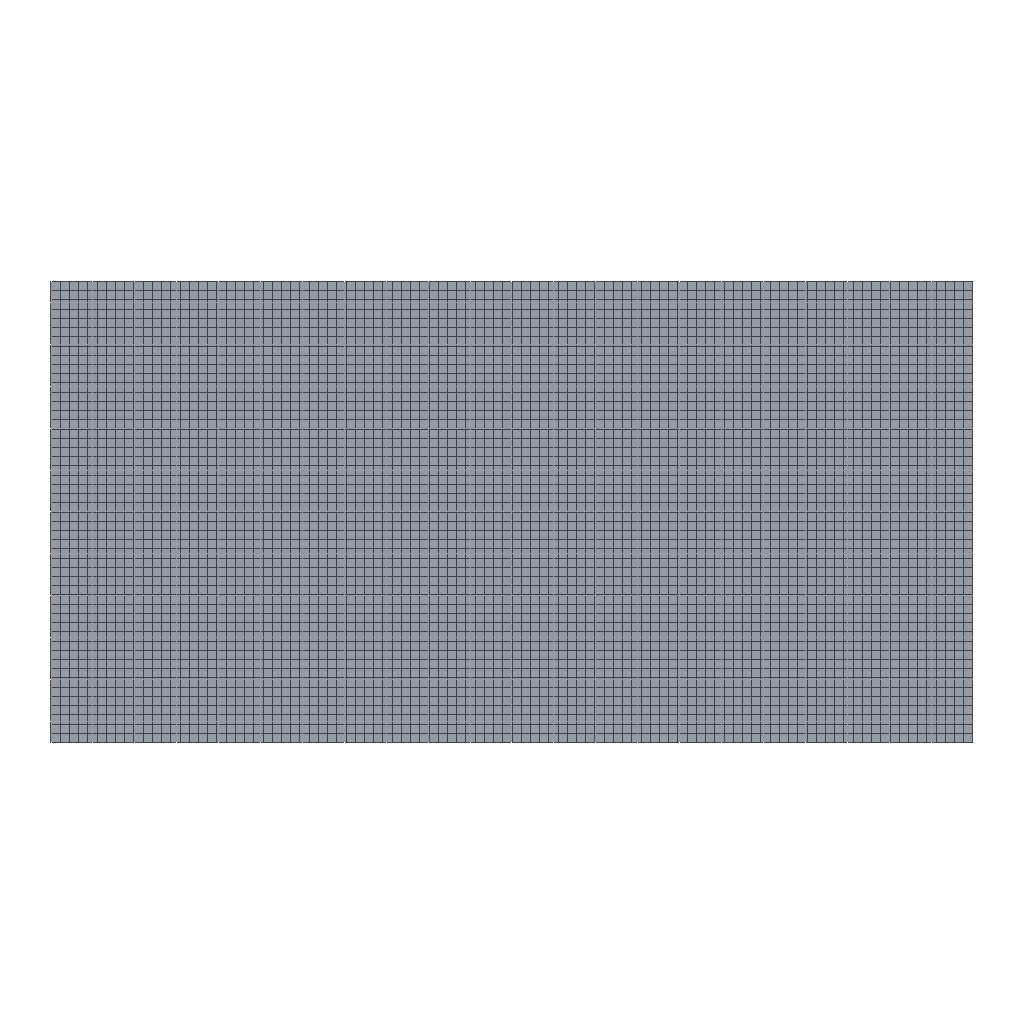Simulation study | abaqus
Set-up summary:
category,name,step,type,value,unit,region
solver,abaqus,,Abaqus/CAE 2024
units,SI m-kg-s (Pa),,inferred,E=1.08e+11 density=4440
analysis,Step-1,,dynamic explicit,nlgeom=True; time_period=0.001075
mesh,nodes,,,5152
mesh,elements,,,5000
element_type,CPE4RT,,,5000
material,TC4,,E,1.08e+11
material,TC4,,nu,0.33
material,TC4,,density,4440
material,TC4,,conductivity,7.5
material,TC4,,cte,9.1e-06
material,TC4,,behaviors,conductivity; damage initiation; damage evolution; expansion
section,TC4,,solid section,,,Set-5
load,Temp,initial,initial condition temperature
bc,BC-1,Step-1,velocity,"-2 [dofs=rz,x,y n=3]",,Set-1
bc,BC-2,Step-1,encastre,[dofs=ENCASTRE],,_PickedSet13
contact,Int-1,Step-1,contact pair,interaction=IntProp-1; friction=0.4; behavior=hard,,tool-1.RigidSurface_ / _PickedSet11_CNS_
constraint,rigid body,,,1
Abaqus input file, long lists of numbers shortened:
*Heading
** Job name: deck Model name: Model-1
** Generated by: Abaqus/CAE 2024
*Preprint, echo=NO, model=NO, history=NO, contact=NO
**
** PARTS
**
*Part, name=tool
*End Part
**
*Part, name=workpiece-mesh-1
*Node
      1, -0.002, -1.92086754e-12
      2, -0.002, -2.00000013e-05
** (5149 more lines like these left out)
*Element, type=CPE4RT
   1,    1,    2,   53,   52
   2,    2,    3,   54,   53
** (4998 more lines like these left out)
*Nset, nset=Set-5, generate
    1,  5151,     1
*Elset, elset=Set-5, generate
    1,  5000,     1
** Section: Section-TC4
*Solid Section, elset=Set-5, controls=EC-1, material=TC4
0.002,
*End Part
**
**
** ASSEMBLY
**
*Assembly, name=Assembly
**
*Instance, name=tool-1, part=tool
9.99999999999998e-05,      -0.0002,           0.
*Node
      1, 0.0006, 0.000975,           0.
*Nset, nset=tool-1-RefPt_, internal
1,
*Surface, type=SEGMENTS, name=RigidSurface_, internal
START,           0.,           0.
 LINE, 0.0006, 6.30625356458706e-05
 LINE, 0.0006,     0.000975
 LINE, 0.0001197,     0.000975
 LINE,           0.,           0.
*End Instance
**
*Instance, name=workpiece-mesh-1-1, part=workpiece-mesh-1
*End Instance
**
*Nset, nset=Set-1, instance=tool-1
 1,
*Nset, nset=_PickedSet11, internal, instance=workpiece-mesh-1-1
    1,    2,    3,    4,    5,    6,    7,    8,    9,   10,   11,   52,   53,   54,   55,   56
   57,   58,   59,   60,   61,   62,  103,  104,  105,  106,  107,  108,  109,  110,  111,  112
** (68 more lines like these left out)
*Nset, nset=_PickedSet13, internal, instance=workpiece-mesh-1-1
    1,    2,    3,    4,    5,    6,    7,    8,    9,   10,   11,   12,   13,   14,   15,   16
   17,   18,   19,   20,   21,   22,   23,   24,   25,   26,   27,   28,   29,   30,   31,   32
** (8 more lines like these left out)
*Nset, nset=_PickedSet14, internal, instance=tool-1
 1,
*Surface, type=NODE, name=_PickedSet11_CNS_, internal
_PickedSet11, 1.
** Constraint: Constraint-1
*Rigid Body, ref node=Set-1, analytical surface=tool-1.RigidSurface_
*End Assembly
**
** ELEMENT CONTROLS
**
*Section Controls, name=EC-1, second order accuracy=YES
1., 1., 1.
*Amplitude, name=Amp-1
             0.,              0.,          0.0001,              1.,          0.0019,              1.,           0.002,              0.
**
** MATERIALS
**
*Material, name=TC4
*Conductivity
  7.5, 20.
  8.7,200.
 11.8,500.
*Damage Initiation, criterion=JOHNSON COOK
 -0.09,  0.25,  -0.5, 0.014,  3.87, 1650.,   25.,    1.
*Damage Evolution, type=DISPLACEMENT
 8e-05,
*Density
4440.,
*Elastic
 1.08e+11, 0.33
*Expansion
 9.1e-06, 20.
 9.2e-06,250.
 9.7e-06,500.
*Inelastic Heat Fraction
         0.9,
*Plastic, hardening=JOHNSON COOK
 8.6e+08, 6.83e+08,     0.47,       1.,    1650.,      25.
*Rate Dependent, type=JOHNSON COOK
 0.035,1.
*Specific Heat
 526.3,
**
** INTERACTION PROPERTIES
**
*Surface Interaction, name=IntProp-1
*Friction
 0.4,
*Surface Behavior, pressure-overclosure=HARD
*Gap Heat Generation
1., 0.5
**
** PREDEFINED FIELDS
**
** Name: Temp works   Type: Temperature
*Initial Conditions, type=TEMPERATURE
_PickedSet14, 298.
** ----------------------------------------------------------------
**
** STEP: Step-1
**
*Step, name=Step-1, nlgeom=YES
*Dynamic, Explicit, adiabatic
, 0.001075
*Bulk Viscosity
0.06, 1.2
** Mass Scaling: Semi-Automatic
**               Whole Model
*Fixed Mass Scaling, factor=200.
**
** BOUNDARY CONDITIONS
**
** Name: BC-1 Type: Velocity/Angular velocity
*Boundary, amplitude=Amp-1, type=VELOCITY
Set-1, 1, 1, -2.
Set-1, 2, 2
Set-1, 6, 6
** Name: BC-2 Type: Symmetry/Antisymmetry/Encastre
*Boundary
_PickedSet13, ENCASTRE
**
** INTERACTIONS
**
** Interaction: Int-1
*Contact Pair, interaction=IntProp-1, mechanical constraint=KINEMATIC, cpset=Int-1
tool-1.RigidSurface_, _PickedSet11_CNS_
**
** OUTPUT REQUESTS
**
*Restart, write, number interval=1, time marks=NO
**
** FIELD OUTPUT: F-Output-1
**
*Output, field, number interval=100
*Node Output
A, RF, U, V
*Element Output, directions=YES
EVF, LE, PE, PEEQ, PEEQVAVG, PEVAVG, S, STATUS, SVAVG
*Contact Output
CSTRESS,
**
** HISTORY OUTPUT: H-Output-1
**
*Output, history, time interval=1.075e-05
*Node Output, nset=Set-1
RF1, RF2, RF3, RM, RM1, RM2, RM3, RT
*End Step
Results summary:
result,odb.job_status,,,JOB_STATUS_COMPLETED_SUCCESSFULLY,"consistent, unstated (Abaqus has no unit system)"
result,steps[0].procedure,cutting,,"*DYNAMIC, EXPLICIT","consistent, unstated (Abaqus has no unit system)"
result,steps[0].time_period,cutting,,0.001075,"consistent, unstated (Abaqus has no unit system)"
result,steps[0].n_frames,cutting,,101,"consistent, unstated (Abaqus has no unit system)"
result,steps[0].last_frame.id,cutting,,76626,"consistent, unstated (Abaqus has no unit system)"
result,steps[0].last_frame.value,cutting,,0.001075,"consistent, unstated (Abaqus has no unit system)"
result,steps[0].last_frame.description,cutting,,Increment     76626: Step Time =   1.0750E-03,"consistent, unstated (Abaqus has no unit system)"
result,steps[0].completed,cutting,,True,"consistent, unstated (Abaqus has no unit system)"
result,steps[0].max_U_magnitude,cutting,,0.02735,"consistent, unstated (Abaqus has no unit system)"
result,steps[0].max_S_mises,cutting,,1.46219e+09,"consistent, unstated (Abaqus has no unit system)"
result,steps[0].RF_sum[1],cutting,,131.815,"consistent, unstated (Abaqus has no unit system)"
result,steps[0].RF_sum[2],cutting,,24.306,"consistent, unstated (Abaqus has no unit system)"
result,steps[0].diagnostic.n_increments,cutting,,101,"consistent, unstated (Abaqus has no unit system)"